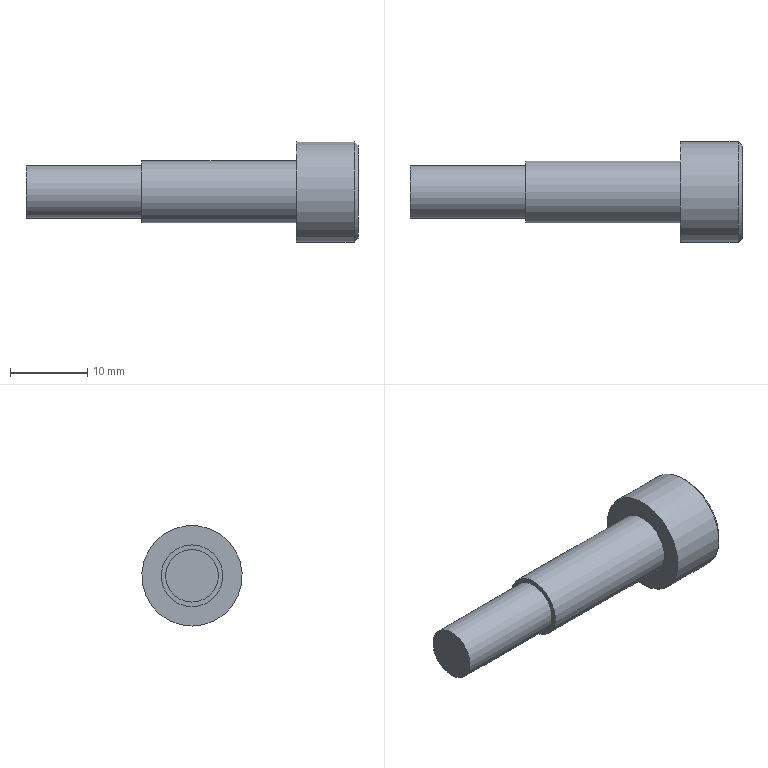Part | STEP file | M3-10_id1366_x_t | 1 solid | 15 faces | box 43 x 13 x 13 mm | volume 2482 mm3 | plane 11 | cylinder 3 | cone 1 | commonest cylinder face diameters 6.8 x1 8 x1 13 x1
STEP:
#1=CARTESIAN_POINT('',(360.,0.,-56.6));
#2=VERTEX_POINT('',#1);
#3=CARTESIAN_POINT('',(360.,0.,-60.));
#4=DIRECTION('',(-1.,0.,0.));
#5=DIRECTION('',(0.,0.,1.));
#6=AXIS2_PLACEMENT_3D('',#3,#4,#5);
#7=CIRCLE('',#6,3.4);
#8=EDGE_CURVE('',#2,#2,#7,.T.);
#9=ORIENTED_EDGE('',*,*,#8,.F.);
#10=EDGE_LOOP('',(#9));
#11=FACE_BOUND('',#10,.T.);
#12=CARTESIAN_POINT('',(360.,0.,-64.));
#13=VERTEX_POINT('',#12);
#14=CARTESIAN_POINT('',(360.,0.,-60.));
#15=DIRECTION('',(1.,0.,0.));
#16=DIRECTION('',(0.,0.,-1.));
#17=AXIS2_PLACEMENT_3D('',#14,#15,#16);
#18=CIRCLE('',#17,4.);
#19=EDGE_CURVE('',#13,#13,#18,.T.);
#20=ORIENTED_EDGE('',*,*,#19,.F.);
#21=EDGE_LOOP('',(#20));
#22=FACE_BOUND('',#21,.T.);
#23=CARTESIAN_POINT('',(360.,0.,-60.));
#24=DIRECTION('',(-1.,0.,0.));
#25=DIRECTION('',(0.,0.,1.));
#26=AXIS2_PLACEMENT_3D('',#23,#24,#25);
#27=PLANE('',#26);
#28=ADVANCED_FACE('',(#11,#22),#27,.T.);
#29=CARTESIAN_POINT('',(380.,0.,-56.));
#30=VERTEX_POINT('',#29);
#31=CARTESIAN_POINT('',(380.,0.,-60.));
#32=DIRECTION('',(1.,0.,0.));
#33=DIRECTION('',(0.,0.,1.));
#34=AXIS2_PLACEMENT_3D('',#31,#32,#33);
#35=CIRCLE('',#34,4.);
#36=EDGE_CURVE('',#30,#30,#35,.T.);
#37=ORIENTED_EDGE('',*,*,#36,.F.);
#38=EDGE_LOOP('',(#37));
#39=FACE_BOUND('',#38,.T.);
#40=ORIENTED_EDGE('',*,*,#19,.T.);
#41=EDGE_LOOP('',(#40));
#42=FACE_BOUND('',#41,.T.);
#43=CARTESIAN_POINT('',(360.,0.,-60.));
#44=DIRECTION('',(1.,0.,0.));
#45=DIRECTION('',(0.,0.,-1.));
#46=AXIS2_PLACEMENT_3D('',#43,#44,#45);
#47=CYLINDRICAL_SURFACE('',#46,4.);
#48=ADVANCED_FACE('',(#39,#42),#47,.T.);
#49=CARTESIAN_POINT('',(345.,0.,-63.4));
#50=VERTEX_POINT('',#49);
#51=CARTESIAN_POINT('',(345.,0.,-60.));
#52=DIRECTION('',(1.,0.,0.));
#53=DIRECTION('',(0.,0.,-1.));
#54=AXIS2_PLACEMENT_3D('',#51,#52,#53);
#55=CIRCLE('',#54,3.4);
#56=EDGE_CURVE('',#50,#50,#55,.T.);
#57=ORIENTED_EDGE('',*,*,#56,.F.);
#58=EDGE_LOOP('',(#57));
#59=FACE_OUTER_BOUND('',#58,.T.);
#60=CARTESIAN_POINT('',(345.,0.,-60.));
#61=DIRECTION('',(-1.,0.,0.));
#62=DIRECTION('',(0.,0.,1.));
#63=AXIS2_PLACEMENT_3D('',#60,#61,#62);
#64=PLANE('',#63);
#65=ADVANCED_FACE('',(#59),#64,.T.);
#66=ORIENTED_EDGE('',*,*,#56,.T.);
#67=EDGE_LOOP('',(#66));
#68=FACE_BOUND('',#67,.T.);
#69=ORIENTED_EDGE('',*,*,#8,.T.);
#70=EDGE_LOOP('',(#69));
#71=FACE_BOUND('',#70,.T.);
#72=CARTESIAN_POINT('',(360.,0.,-60.));
#73=DIRECTION('',(-1.,0.,0.));
#74=DIRECTION('',(0.,0.,-1.));
#75=AXIS2_PLACEMENT_3D('',#72,#73,#74);
#76=CYLINDRICAL_SURFACE('',#75,3.4);
#77=ADVANCED_FACE('',(#68,#71),#76,.T.);
#78=CARTESIAN_POINT('',(388.,1.732,-57.));
#79=VERTEX_POINT('',#78);
#80=CARTESIAN_POINT('',(388.,-1.732,-57.));
#81=VERTEX_POINT('',#80);
#82=CARTESIAN_POINT('',(388.,1.732,-57.));
#83=DIRECTION('',(0.,-1.,0.));
#84=VECTOR('',#83,1.);
#85=LINE('',#82,#84);
#86=EDGE_CURVE('',#79,#81,#85,.T.);
#87=ORIENTED_EDGE('',*,*,#86,.F.);
#88=CARTESIAN_POINT('',(388.,3.464,-60.));
#89=VERTEX_POINT('',#88);
#90=CARTESIAN_POINT('',(388.,3.464,-60.));
#91=DIRECTION('',(0.,-0.5,0.866));
#92=VECTOR('',#91,1.);
#93=LINE('',#90,#92);
#94=EDGE_CURVE('',#89,#79,#93,.T.);
#95=ORIENTED_EDGE('',*,*,#94,.F.);
#96=CARTESIAN_POINT('',(388.,1.732,-63.));
#97=VERTEX_POINT('',#96);
#98=CARTESIAN_POINT('',(388.,1.732,-63.));
#99=DIRECTION('',(0.,0.5,0.866));
#100=VECTOR('',#99,1.);
#101=LINE('',#98,#100);
#102=EDGE_CURVE('',#97,#89,#101,.T.);
#103=ORIENTED_EDGE('',*,*,#102,.F.);
#104=CARTESIAN_POINT('',(388.,-1.732,-63.));
#105=VERTEX_POINT('',#104);
#106=CARTESIAN_POINT('',(388.,-1.732,-63.));
#107=DIRECTION('',(0.,1.,0.));
#108=VECTOR('',#107,1.);
#109=LINE('',#106,#108);
#110=EDGE_CURVE('',#105,#97,#109,.T.);
#111=ORIENTED_EDGE('',*,*,#110,.F.);
#112=CARTESIAN_POINT('',(388.,-3.464,-60.));
#113=VERTEX_POINT('',#112);
#114=CARTESIAN_POINT('',(388.,-3.464,-60.));
#115=DIRECTION('',(0.,0.5,-0.866));
#116=VECTOR('',#115,1.);
#117=LINE('',#114,#116);
#118=EDGE_CURVE('',#113,#105,#117,.T.);
#119=ORIENTED_EDGE('',*,*,#118,.F.);
#120=CARTESIAN_POINT('',(388.,-1.732,-57.));
#121=DIRECTION('',(0.,-0.5,-0.866));
#122=VECTOR('',#121,1.);
#123=LINE('',#120,#122);
#124=EDGE_CURVE('',#81,#113,#123,.T.);
#125=ORIENTED_EDGE('',*,*,#124,.F.);
#126=EDGE_LOOP('',(#87,#95,#103,#111,#119,#125));
#127=FACE_BOUND('',#126,.T.);
#128=CARTESIAN_POINT('',(388.,0.,-66.));
#129=VERTEX_POINT('',#128);
#130=CARTESIAN_POINT('',(388.,0.,-60.));
#131=DIRECTION('',(1.,0.,0.));
#132=DIRECTION('',(0.,0.,-1.));
#133=AXIS2_PLACEMENT_3D('',#130,#131,#132);
#134=CIRCLE('',#133,6.);
#135=EDGE_CURVE('',#129,#129,#134,.T.);
#136=ORIENTED_EDGE('',*,*,#135,.T.);
#137=EDGE_LOOP('',(#136));
#138=FACE_BOUND('',#137,.T.);
#139=CARTESIAN_POINT('',(388.,0.,-60.));
#140=DIRECTION('',(1.,0.,0.));
#141=DIRECTION('',(0.,0.,-1.));
#142=AXIS2_PLACEMENT_3D('',#139,#140,#141);
#143=PLANE('',#142);
#144=ADVANCED_FACE('',(#127,#138),#143,.T.);
#145=ORIENTED_EDGE('',*,*,#36,.T.);
#146=EDGE_LOOP('',(#145));
#147=FACE_BOUND('',#146,.T.);
#148=CARTESIAN_POINT('',(380.,0.,-66.5));
#149=VERTEX_POINT('',#148);
#150=CARTESIAN_POINT('',(380.,0.,-60.));
#151=DIRECTION('',(1.,0.,0.));
#152=DIRECTION('',(0.,0.,-1.));
#153=AXIS2_PLACEMENT_3D('',#150,#151,#152);
#154=CIRCLE('',#153,6.5);
#155=EDGE_CURVE('',#149,#149,#154,.T.);
#156=ORIENTED_EDGE('',*,*,#155,.F.);
#157=EDGE_LOOP('',(#156));
#158=FACE_BOUND('',#157,.T.);
#159=CARTESIAN_POINT('',(380.,0.,-60.));
#160=DIRECTION('',(-1.,0.,0.));
#161=DIRECTION('',(0.,0.,1.));
#162=AXIS2_PLACEMENT_3D('',#159,#160,#161);
#163=PLANE('',#162);
#164=ADVANCED_FACE('',(#147,#158),#163,.T.);
#165=CARTESIAN_POINT('',(387.5,0.,-66.5));
#166=VERTEX_POINT('',#165);
#167=CARTESIAN_POINT('',(387.5,0.,-60.));
#168=DIRECTION('',(-1.,0.,0.));
#169=DIRECTION('',(0.,0.,-1.));
#170=AXIS2_PLACEMENT_3D('',#167,#168,#169);
#171=CIRCLE('',#170,6.5);
#172=EDGE_CURVE('',#166,#166,#171,.T.);
#173=ORIENTED_EDGE('',*,*,#172,.T.);
#174=EDGE_LOOP('',(#173));
#175=FACE_BOUND('',#174,.T.);
#176=ORIENTED_EDGE('',*,*,#155,.T.);
#177=EDGE_LOOP('',(#176));
#178=FACE_BOUND('',#177,.T.);
#179=CARTESIAN_POINT('',(380.,0.,-60.));
#180=DIRECTION('',(1.,0.,0.));
#181=DIRECTION('',(0.,0.,-1.));
#182=AXIS2_PLACEMENT_3D('',#179,#180,#181);
#183=CYLINDRICAL_SURFACE('',#182,6.5);
#184=ADVANCED_FACE('',(#175,#178),#183,.T.);
#185=ORIENTED_EDGE('',*,*,#135,.F.);
#186=EDGE_LOOP('',(#185));
#187=FACE_BOUND('',#186,.T.);
#188=ORIENTED_EDGE('',*,*,#172,.F.);
#189=EDGE_LOOP('',(#188));
#190=FACE_BOUND('',#189,.T.);
#191=CARTESIAN_POINT('',(387.5,0.,-60.));
#192=DIRECTION('',(-1.,0.,0.));
#193=DIRECTION('',(0.,0.,1.));
#194=AXIS2_PLACEMENT_3D('',#191,#192,#193);
#195=CONICAL_SURFACE('',#194,6.5,45.);
#196=ADVANCED_FACE('',(#187,#190),#195,.T.);
#197=ORIENTED_EDGE('',*,*,#86,.T.);
#198=CARTESIAN_POINT('',(384.,-1.732,-57.));
#199=VERTEX_POINT('',#198);
#200=CARTESIAN_POINT('',(384.,-1.732,-57.));
#201=DIRECTION('',(-1.,0.,0.));
#202=VECTOR('',#201,1.);
#203=LINE('',#200,#202);
#204=EDGE_CURVE('',#81,#199,#203,.T.);
#205=ORIENTED_EDGE('',*,*,#204,.T.);
#206=CARTESIAN_POINT('',(384.,1.732,-57.));
#207=VERTEX_POINT('',#206);
#208=CARTESIAN_POINT('',(384.,1.732,-57.));
#209=DIRECTION('',(0.,1.,0.));
#210=VECTOR('',#209,1.);
#211=LINE('',#208,#210);
#212=EDGE_CURVE('',#199,#207,#211,.T.);
#213=ORIENTED_EDGE('',*,*,#212,.T.);
#214=CARTESIAN_POINT('',(384.,1.732,-57.));
#215=DIRECTION('',(-1.,0.,0.));
#216=VECTOR('',#215,1.);
#217=LINE('',#214,#216);
#218=EDGE_CURVE('',#79,#207,#217,.T.);
#219=ORIENTED_EDGE('',*,*,#218,.F.);
#220=EDGE_LOOP('',(#197,#205,#213,#219));
#221=FACE_OUTER_BOUND('',#220,.T.);
#222=CARTESIAN_POINT('',(384.,1.732,-57.));
#223=DIRECTION('',(0.,0.,1.));
#224=DIRECTION('',(1.,0.,0.));
#225=AXIS2_PLACEMENT_3D('',#222,#223,#224);
#226=PLANE('',#225);
#227=ADVANCED_FACE('',(#221),#226,.F.);
#228=ORIENTED_EDGE('',*,*,#124,.T.);
#229=CARTESIAN_POINT('',(384.,-3.464,-60.));
#230=VERTEX_POINT('',#229);
#231=CARTESIAN_POINT('',(384.,-3.464,-60.));
#232=DIRECTION('',(-1.,0.,0.));
#233=VECTOR('',#232,1.);
#234=LINE('',#231,#233);
#235=EDGE_CURVE('',#113,#230,#234,.T.);
#236=ORIENTED_EDGE('',*,*,#235,.T.);
#237=CARTESIAN_POINT('',(384.,-1.732,-57.));
#238=DIRECTION('',(0.,0.5,0.866));
#239=VECTOR('',#238,1.);
#240=LINE('',#237,#239);
#241=EDGE_CURVE('',#230,#199,#240,.T.);
#242=ORIENTED_EDGE('',*,*,#241,.T.);
#243=ORIENTED_EDGE('',*,*,#204,.F.);
#244=EDGE_LOOP('',(#228,#236,#242,#243));
#245=FACE_OUTER_BOUND('',#244,.T.);
#246=CARTESIAN_POINT('',(384.,-1.732,-57.));
#247=DIRECTION('',(0.,-0.866,0.5));
#248=DIRECTION('',(0.,-0.5,-0.866));
#249=AXIS2_PLACEMENT_3D('',#246,#247,#248);
#250=PLANE('',#249);
#251=ADVANCED_FACE('',(#245),#250,.F.);
#252=ORIENTED_EDGE('',*,*,#118,.T.);
#253=CARTESIAN_POINT('',(384.,-1.732,-63.));
#254=VERTEX_POINT('',#253);
#255=CARTESIAN_POINT('',(384.,-1.732,-63.));
#256=DIRECTION('',(-1.,0.,0.));
#257=VECTOR('',#256,1.);
#258=LINE('',#255,#257);
#259=EDGE_CURVE('',#105,#254,#258,.T.);
#260=ORIENTED_EDGE('',*,*,#259,.T.);
#261=CARTESIAN_POINT('',(384.,-3.464,-60.));
#262=DIRECTION('',(0.,-0.5,0.866));
#263=VECTOR('',#262,1.);
#264=LINE('',#261,#263);
#265=EDGE_CURVE('',#254,#230,#264,.T.);
#266=ORIENTED_EDGE('',*,*,#265,.T.);
#267=ORIENTED_EDGE('',*,*,#235,.F.);
#268=EDGE_LOOP('',(#252,#260,#266,#267));
#269=FACE_OUTER_BOUND('',#268,.T.);
#270=CARTESIAN_POINT('',(384.,-3.464,-60.));
#271=DIRECTION('',(0.,-0.866,-0.5));
#272=DIRECTION('',(0.,0.5,-0.866));
#273=AXIS2_PLACEMENT_3D('',#270,#271,#272);
#274=PLANE('',#273);
#275=ADVANCED_FACE('',(#269),#274,.F.);
#276=ORIENTED_EDGE('',*,*,#110,.T.);
#277=CARTESIAN_POINT('',(384.,1.732,-63.));
#278=VERTEX_POINT('',#277);
#279=CARTESIAN_POINT('',(384.,1.732,-63.));
#280=DIRECTION('',(-1.,0.,0.));
#281=VECTOR('',#280,1.);
#282=LINE('',#279,#281);
#283=EDGE_CURVE('',#97,#278,#282,.T.);
#284=ORIENTED_EDGE('',*,*,#283,.T.);
#285=CARTESIAN_POINT('',(384.,-1.732,-63.));
#286=DIRECTION('',(0.,-1.,0.));
#287=VECTOR('',#286,1.);
#288=LINE('',#285,#287);
#289=EDGE_CURVE('',#278,#254,#288,.T.);
#290=ORIENTED_EDGE('',*,*,#289,.T.);
#291=ORIENTED_EDGE('',*,*,#259,.F.);
#292=EDGE_LOOP('',(#276,#284,#290,#291));
#293=FACE_OUTER_BOUND('',#292,.T.);
#294=CARTESIAN_POINT('',(384.,-1.732,-63.));
#295=DIRECTION('',(0.,0.,-1.));
#296=DIRECTION('',(0.,1.,0.));
#297=AXIS2_PLACEMENT_3D('',#294,#295,#296);
#298=PLANE('',#297);
#299=ADVANCED_FACE('',(#293),#298,.F.);
#300=ORIENTED_EDGE('',*,*,#102,.T.);
#301=CARTESIAN_POINT('',(384.,3.464,-60.));
#302=VERTEX_POINT('',#301);
#303=CARTESIAN_POINT('',(384.,3.464,-60.));
#304=DIRECTION('',(-1.,0.,0.));
#305=VECTOR('',#304,1.);
#306=LINE('',#303,#305);
#307=EDGE_CURVE('',#89,#302,#306,.T.);
#308=ORIENTED_EDGE('',*,*,#307,.T.);
#309=CARTESIAN_POINT('',(384.,1.732,-63.));
#310=DIRECTION('',(0.,-0.5,-0.866));
#311=VECTOR('',#310,1.);
#312=LINE('',#309,#311);
#313=EDGE_CURVE('',#302,#278,#312,.T.);
#314=ORIENTED_EDGE('',*,*,#313,.T.);
#315=ORIENTED_EDGE('',*,*,#283,.F.);
#316=EDGE_LOOP('',(#300,#308,#314,#315));
#317=FACE_OUTER_BOUND('',#316,.T.);
#318=CARTESIAN_POINT('',(384.,1.732,-63.));
#319=DIRECTION('',(0.,0.866,-0.5));
#320=DIRECTION('',(0.,0.5,0.866));
#321=AXIS2_PLACEMENT_3D('',#318,#319,#320);
#322=PLANE('',#321);
#323=ADVANCED_FACE('',(#317),#322,.F.);
#324=ORIENTED_EDGE('',*,*,#94,.T.);
#325=ORIENTED_EDGE('',*,*,#218,.T.);
#326=CARTESIAN_POINT('',(384.,3.464,-60.));
#327=DIRECTION('',(0.,0.5,-0.866));
#328=VECTOR('',#327,1.);
#329=LINE('',#326,#328);
#330=EDGE_CURVE('',#207,#302,#329,.T.);
#331=ORIENTED_EDGE('',*,*,#330,.T.);
#332=ORIENTED_EDGE('',*,*,#307,.F.);
#333=EDGE_LOOP('',(#324,#325,#331,#332));
#334=FACE_OUTER_BOUND('',#333,.T.);
#335=CARTESIAN_POINT('',(384.,3.464,-60.));
#336=DIRECTION('',(0.,0.866,0.5));
#337=DIRECTION('',(0.,-0.5,0.866));
#338=AXIS2_PLACEMENT_3D('',#335,#336,#337);
#339=PLANE('',#338);
#340=ADVANCED_FACE('',(#334),#339,.F.);
#341=ORIENTED_EDGE('',*,*,#212,.F.);
#342=ORIENTED_EDGE('',*,*,#241,.F.);
#343=ORIENTED_EDGE('',*,*,#265,.F.);
#344=ORIENTED_EDGE('',*,*,#289,.F.);
#345=ORIENTED_EDGE('',*,*,#313,.F.);
#346=ORIENTED_EDGE('',*,*,#330,.F.);
#347=EDGE_LOOP('',(#341,#342,#343,#344,#345,#346));
#348=FACE_OUTER_BOUND('',#347,.T.);
#349=CARTESIAN_POINT('',(384.,0.,-60.));
#350=DIRECTION('',(1.,0.,0.));
#351=DIRECTION('',(0.,0.,-1.));
#352=AXIS2_PLACEMENT_3D('',#349,#350,#351);
#353=PLANE('',#352);
#354=ADVANCED_FACE('',(#348),#353,.T.);
#355=CLOSED_SHELL('',(#28,#48,#65,#77,#144,#164,#184,#196,#227,#251,#275,#299,#323,#340,#354));
#356=MANIFOLD_SOLID_BREP('',#355);
#357=(LENGTH_UNIT()NAMED_UNIT(*)SI_UNIT(.MILLI.,.METRE.));
#358=UNCERTAINTY_MEASURE_WITH_UNIT(LENGTH_MEASURE(0.00002),#357,'','');
#359=(NAMED_UNIT(*)PLANE_ANGLE_UNIT()SI_UNIT($,.RADIAN.));
#360=PLANE_ANGLE_MEASURE_WITH_UNIT(PLANE_ANGLE_MEASURE(0.01745),#359);
#361=DIMENSIONAL_EXPONENTS(0.,0.,0.,0.,0.,0.,0.);
#362=(CONVERSION_BASED_UNIT('DEGREE',#360)NAMED_UNIT(#361)PLANE_ANGLE_UNIT());
#363=(NAMED_UNIT(*)SI_UNIT($,.STERADIAN.)SOLID_ANGLE_UNIT());
#364=(GEOMETRIC_REPRESENTATION_CONTEXT(3)GLOBAL_UNCERTAINTY_ASSIGNED_CONTEXT((#358))GLOBAL_UNIT_ASSIGNED_CONTEXT((#357,#362,#363))REPRESENTATION_CONTEXT('',''));
#365=ADVANCED_BREP_SHAPE_REPRESENTATION('',(#356),#364);